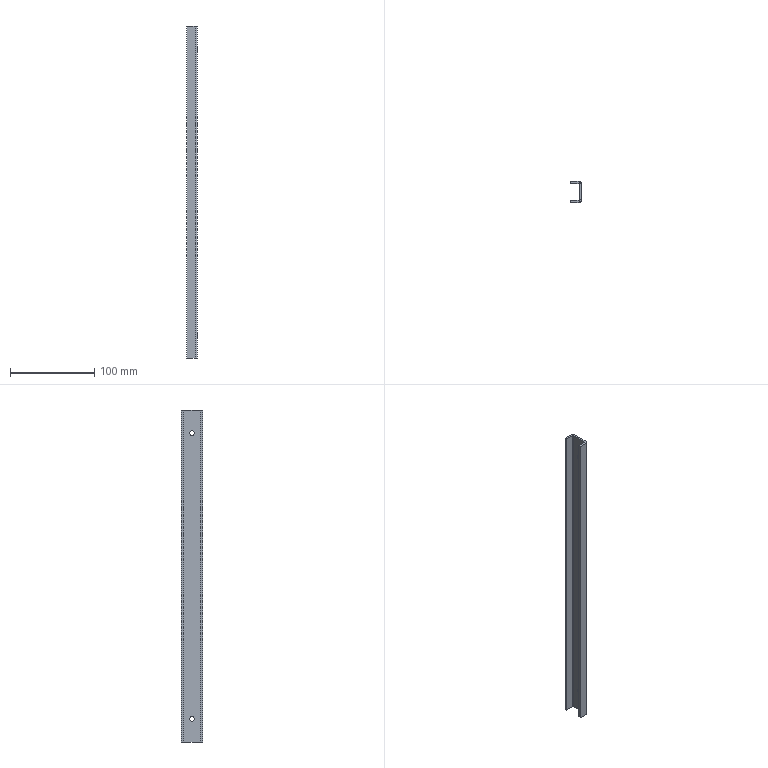Part | SolidWorks | features Cut 1, FlatPattern 1, SMBaseFlange 1, SheetMetal 1 | 1 solid | 26 faces | box 13 x 25 x 395 mm | volume 44005 mm3 | plane 18 | cylinder 8 | commonest cylinder face diameters 5.2 x4 0.6 x2 5.6 x2
STEP:
#1=CARTESIAN_POINT('',(10.5,12.5,30.1));
#2=VERTEX_POINT('',#1);
#3=CARTESIAN_POINT('',(10.5,12.5,24.9));
#4=VERTEX_POINT('',#3);
#5=CARTESIAN_POINT('',(10.5,12.5,27.5));
#6=DIRECTION('',(1.,0.,0.));
#7=DIRECTION('',(0.,0.,-1.));
#8=AXIS2_PLACEMENT_3D('',#5,#6,#7);
#9=CIRCLE('',#8,2.6);
#10=EDGE_CURVE('',#2,#4,#9,.T.);
#11=ORIENTED_EDGE('',*,*,#10,.F.);
#12=CARTESIAN_POINT('',(13.,12.5,30.1));
#13=VERTEX_POINT('',#12);
#14=CARTESIAN_POINT('',(10.5,12.5,30.1));
#15=DIRECTION('',(1.,0.,0.));
#16=VECTOR('',#15,1000.);
#17=LINE('',#14,#16);
#18=EDGE_CURVE('',#2,#13,#17,.T.);
#19=ORIENTED_EDGE('',*,*,#18,.T.);
#20=CARTESIAN_POINT('',(13.,12.5,24.9));
#21=VERTEX_POINT('',#20);
#22=CARTESIAN_POINT('',(13.,12.5,27.5));
#23=DIRECTION('',(1.,0.,0.));
#24=DIRECTION('',(0.,0.,-1.));
#25=AXIS2_PLACEMENT_3D('',#22,#23,#24);
#26=CIRCLE('',#25,2.6);
#27=EDGE_CURVE('',#13,#21,#26,.T.);
#28=ORIENTED_EDGE('',*,*,#27,.T.);
#29=CARTESIAN_POINT('',(10.5,12.5,24.9));
#30=DIRECTION('',(1.,0.,0.));
#31=VECTOR('',#30,1000.);
#32=LINE('',#29,#31);
#33=EDGE_CURVE('',#4,#21,#32,.T.);
#34=ORIENTED_EDGE('',*,*,#33,.F.);
#35=EDGE_LOOP('',(#11,#19,#28,#34));
#36=FACE_OUTER_BOUND('',#35,.T.);
#37=CARTESIAN_POINT('',(10.5,12.5,27.5));
#38=DIRECTION('',(1.,0.,0.));
#39=DIRECTION('',(0.,0.,-1.));
#40=AXIS2_PLACEMENT_3D('',#37,#38,#39);
#41=CYLINDRICAL_SURFACE('',#40,2.6);
#42=ADVANCED_FACE('',(#36),#41,.F.);
#43=CARTESIAN_POINT('',(10.5,12.5,370.1));
#44=VERTEX_POINT('',#43);
#45=CARTESIAN_POINT('',(10.5,12.5,364.9));
#46=VERTEX_POINT('',#45);
#47=CARTESIAN_POINT('',(10.5,12.5,367.5));
#48=DIRECTION('',(1.,0.,0.));
#49=DIRECTION('',(0.,0.,-1.));
#50=AXIS2_PLACEMENT_3D('',#47,#48,#49);
#51=CIRCLE('',#50,2.6);
#52=EDGE_CURVE('',#44,#46,#51,.T.);
#53=ORIENTED_EDGE('',*,*,#52,.F.);
#54=CARTESIAN_POINT('',(13.,12.5,370.1));
#55=VERTEX_POINT('',#54);
#56=CARTESIAN_POINT('',(10.5,12.5,370.1));
#57=DIRECTION('',(1.,0.,0.));
#58=VECTOR('',#57,1000.);
#59=LINE('',#56,#58);
#60=EDGE_CURVE('',#44,#55,#59,.T.);
#61=ORIENTED_EDGE('',*,*,#60,.T.);
#62=CARTESIAN_POINT('',(13.,12.5,364.9));
#63=VERTEX_POINT('',#62);
#64=CARTESIAN_POINT('',(13.,12.5,367.5));
#65=DIRECTION('',(1.,0.,0.));
#66=DIRECTION('',(0.,0.,-1.));
#67=AXIS2_PLACEMENT_3D('',#64,#65,#66);
#68=CIRCLE('',#67,2.6);
#69=EDGE_CURVE('',#55,#63,#68,.T.);
#70=ORIENTED_EDGE('',*,*,#69,.T.);
#71=CARTESIAN_POINT('',(10.5,12.5,364.9));
#72=DIRECTION('',(1.,0.,0.));
#73=VECTOR('',#72,1000.);
#74=LINE('',#71,#73);
#75=EDGE_CURVE('',#46,#63,#74,.T.);
#76=ORIENTED_EDGE('',*,*,#75,.F.);
#77=EDGE_LOOP('',(#53,#61,#70,#76));
#78=FACE_OUTER_BOUND('',#77,.T.);
#79=CARTESIAN_POINT('',(10.5,12.5,367.5));
#80=DIRECTION('',(1.,0.,0.));
#81=DIRECTION('',(0.,0.,-1.));
#82=AXIS2_PLACEMENT_3D('',#79,#80,#81);
#83=CYLINDRICAL_SURFACE('',#82,2.6);
#84=ADVANCED_FACE('',(#78),#83,.F.);
#85=CARTESIAN_POINT('',(10.2,0.,395.));
#86=VERTEX_POINT('',#85);
#87=CARTESIAN_POINT('',(10.2,2.5,395.));
#88=VERTEX_POINT('',#87);
#89=CARTESIAN_POINT('',(10.2,0.,395.));
#90=DIRECTION('',(0.,1.,0.));
#91=VECTOR('',#90,1000.);
#92=LINE('',#89,#91);
#93=EDGE_CURVE('',#86,#88,#92,.T.);
#94=ORIENTED_EDGE('',*,*,#93,.F.);
#95=CARTESIAN_POINT('',(13.,2.8,395.));
#96=VERTEX_POINT('',#95);
#97=CARTESIAN_POINT('',(10.2,2.8,395.));
#98=DIRECTION('',(0.,0.,1.));
#99=DIRECTION('',(-1.,0.,0.));
#100=AXIS2_PLACEMENT_3D('',#97,#98,#99);
#101=CIRCLE('',#100,2.8);
#102=EDGE_CURVE('',#86,#96,#101,.T.);
#103=ORIENTED_EDGE('',*,*,#102,.T.);
#104=CARTESIAN_POINT('',(10.5,2.8,395.));
#105=VERTEX_POINT('',#104);
#106=CARTESIAN_POINT('',(10.5,2.8,395.));
#107=DIRECTION('',(1.,0.,0.));
#108=VECTOR('',#107,1000.);
#109=LINE('',#106,#108);
#110=EDGE_CURVE('',#105,#96,#109,.T.);
#111=ORIENTED_EDGE('',*,*,#110,.F.);
#112=CARTESIAN_POINT('',(10.2,2.8,395.));
#113=DIRECTION('',(0.,0.,1.));
#114=DIRECTION('',(1.,0.,0.));
#115=AXIS2_PLACEMENT_3D('',#112,#113,#114);
#116=CIRCLE('',#115,0.3);
#117=EDGE_CURVE('',#88,#105,#116,.T.);
#118=ORIENTED_EDGE('',*,*,#117,.F.);
#119=EDGE_LOOP('',(#94,#103,#111,#118));
#120=FACE_OUTER_BOUND('',#119,.T.);
#121=CARTESIAN_POINT('',(10.2,0.,395.));
#122=DIRECTION('',(0.,0.,1.));
#123=DIRECTION('',(1.,0.,0.));
#124=AXIS2_PLACEMENT_3D('',#121,#122,#123);
#125=PLANE('',#124);
#126=ADVANCED_FACE('',(#120),#125,.T.);
#127=CARTESIAN_POINT('',(0.,0.,395.));
#128=VERTEX_POINT('',#127);
#129=CARTESIAN_POINT('',(0.,0.,395.));
#130=DIRECTION('',(1.,0.,0.));
#131=VECTOR('',#130,1000.);
#132=LINE('',#129,#131);
#133=EDGE_CURVE('',#128,#86,#132,.T.);
#134=ORIENTED_EDGE('',*,*,#133,.T.);
#135=ORIENTED_EDGE('',*,*,#93,.T.);
#136=CARTESIAN_POINT('',(0.,2.5,395.));
#137=VERTEX_POINT('',#136);
#138=CARTESIAN_POINT('',(0.,2.5,395.));
#139=DIRECTION('',(1.,0.,0.));
#140=VECTOR('',#139,1000.);
#141=LINE('',#138,#140);
#142=EDGE_CURVE('',#137,#88,#141,.T.);
#143=ORIENTED_EDGE('',*,*,#142,.F.);
#144=CARTESIAN_POINT('',(0.,0.,395.));
#145=DIRECTION('',(0.,1.,0.));
#146=VECTOR('',#145,1000.);
#147=LINE('',#144,#146);
#148=EDGE_CURVE('',#128,#137,#147,.T.);
#149=ORIENTED_EDGE('',*,*,#148,.F.);
#150=EDGE_LOOP('',(#134,#135,#143,#149));
#151=FACE_OUTER_BOUND('',#150,.T.);
#152=CARTESIAN_POINT('',(10.5,2.8,395.));
#153=DIRECTION('',(0.,0.,1.));
#154=DIRECTION('',(1.,0.,0.));
#155=AXIS2_PLACEMENT_3D('',#152,#153,#154);
#156=PLANE('',#155);
#157=ADVANCED_FACE('',(#151),#156,.T.);
#158=CARTESIAN_POINT('',(13.,2.8,0.));
#159=VERTEX_POINT('',#158);
#160=CARTESIAN_POINT('',(10.5,2.8,0.));
#161=VERTEX_POINT('',#160);
#162=CARTESIAN_POINT('',(13.,2.8,0.));
#163=DIRECTION('',(-1.,0.,0.));
#164=VECTOR('',#163,1000.);
#165=LINE('',#162,#164);
#166=EDGE_CURVE('',#159,#161,#165,.T.);
#167=ORIENTED_EDGE('',*,*,#166,.F.);
#168=CARTESIAN_POINT('',(10.2,0.,0.));
#169=VERTEX_POINT('',#168);
#170=CARTESIAN_POINT('',(10.2,2.8,0.));
#171=DIRECTION('',(0.,0.,1.));
#172=DIRECTION('',(-1.,0.,0.));
#173=AXIS2_PLACEMENT_3D('',#170,#171,#172);
#174=CIRCLE('',#173,2.8);
#175=EDGE_CURVE('',#169,#159,#174,.T.);
#176=ORIENTED_EDGE('',*,*,#175,.F.);
#177=CARTESIAN_POINT('',(10.2,2.5,0.));
#178=VERTEX_POINT('',#177);
#179=CARTESIAN_POINT('',(10.2,2.5,0.));
#180=DIRECTION('',(0.,-1.,0.));
#181=VECTOR('',#180,1000.);
#182=LINE('',#179,#181);
#183=EDGE_CURVE('',#178,#169,#182,.T.);
#184=ORIENTED_EDGE('',*,*,#183,.F.);
#185=CARTESIAN_POINT('',(10.2,2.8,0.));
#186=DIRECTION('',(0.,0.,1.));
#187=DIRECTION('',(1.,0.,0.));
#188=AXIS2_PLACEMENT_3D('',#185,#186,#187);
#189=CIRCLE('',#188,0.3);
#190=EDGE_CURVE('',#178,#161,#189,.T.);
#191=ORIENTED_EDGE('',*,*,#190,.T.);
#192=EDGE_LOOP('',(#167,#176,#184,#191));
#193=FACE_OUTER_BOUND('',#192,.T.);
#194=CARTESIAN_POINT('',(13.,2.8,0.));
#195=DIRECTION('',(0.,0.,-1.));
#196=DIRECTION('',(-1.,0.,0.));
#197=AXIS2_PLACEMENT_3D('',#194,#195,#196);
#198=PLANE('',#197);
#199=ADVANCED_FACE('',(#193),#198,.T.);
#200=CARTESIAN_POINT('',(13.,22.2,0.));
#201=VERTEX_POINT('',#200);
#202=CARTESIAN_POINT('',(13.,0.,0.));
#203=DIRECTION('',(0.,1.,0.));
#204=VECTOR('',#203,1000.);
#205=LINE('',#202,#204);
#206=EDGE_CURVE('',#159,#201,#205,.T.);
#207=ORIENTED_EDGE('',*,*,#206,.F.);
#208=ORIENTED_EDGE('',*,*,#166,.T.);
#209=CARTESIAN_POINT('',(10.5,22.2,0.));
#210=VERTEX_POINT('',#209);
#211=CARTESIAN_POINT('',(10.5,0.,0.));
#212=DIRECTION('',(0.,1.,0.));
#213=VECTOR('',#212,1000.);
#214=LINE('',#211,#213);
#215=EDGE_CURVE('',#161,#210,#214,.T.);
#216=ORIENTED_EDGE('',*,*,#215,.T.);
#217=CARTESIAN_POINT('',(10.5,22.2,0.));
#218=DIRECTION('',(1.,0.,0.));
#219=VECTOR('',#218,1000.);
#220=LINE('',#217,#219);
#221=EDGE_CURVE('',#210,#201,#220,.T.);
#222=ORIENTED_EDGE('',*,*,#221,.T.);
#223=EDGE_LOOP('',(#207,#208,#216,#222));
#224=FACE_OUTER_BOUND('',#223,.T.);
#225=CARTESIAN_POINT('',(10.2,2.5,0.));
#226=DIRECTION('',(0.,0.,-1.));
#227=DIRECTION('',(-1.,0.,0.));
#228=AXIS2_PLACEMENT_3D('',#225,#226,#227);
#229=PLANE('',#228);
#230=ADVANCED_FACE('',(#224),#229,.T.);
#231=CARTESIAN_POINT('',(13.,22.2,395.));
#232=VERTEX_POINT('',#231);
#233=CARTESIAN_POINT('',(10.5,22.2,395.));
#234=VERTEX_POINT('',#233);
#235=CARTESIAN_POINT('',(13.,22.2,395.));
#236=DIRECTION('',(-1.,0.,0.));
#237=VECTOR('',#236,1000.);
#238=LINE('',#235,#237);
#239=EDGE_CURVE('',#232,#234,#238,.T.);
#240=ORIENTED_EDGE('',*,*,#239,.F.);
#241=CARTESIAN_POINT('',(10.2,25.,395.));
#242=VERTEX_POINT('',#241);
#243=CARTESIAN_POINT('',(10.2,22.2,395.));
#244=DIRECTION('',(0.,0.,1.));
#245=DIRECTION('',(-1.,0.,0.));
#246=AXIS2_PLACEMENT_3D('',#243,#244,#245);
#247=CIRCLE('',#246,2.8);
#248=EDGE_CURVE('',#232,#242,#247,.T.);
#249=ORIENTED_EDGE('',*,*,#248,.T.);
#250=CARTESIAN_POINT('',(10.2,22.5,395.));
#251=VERTEX_POINT('',#250);
#252=CARTESIAN_POINT('',(10.2,22.5,395.));
#253=DIRECTION('',(0.,1.,0.));
#254=VECTOR('',#253,1000.);
#255=LINE('',#252,#254);
#256=EDGE_CURVE('',#251,#242,#255,.T.);
#257=ORIENTED_EDGE('',*,*,#256,.F.);
#258=CARTESIAN_POINT('',(10.2,22.2,395.));
#259=DIRECTION('',(0.,0.,1.));
#260=DIRECTION('',(1.,0.,0.));
#261=AXIS2_PLACEMENT_3D('',#258,#259,#260);
#262=CIRCLE('',#261,0.3);
#263=EDGE_CURVE('',#234,#251,#262,.T.);
#264=ORIENTED_EDGE('',*,*,#263,.F.);
#265=EDGE_LOOP('',(#240,#249,#257,#264));
#266=FACE_OUTER_BOUND('',#265,.T.);
#267=CARTESIAN_POINT('',(13.,22.2,395.));
#268=DIRECTION('',(0.,0.,1.));
#269=DIRECTION('',(1.,0.,0.));
#270=AXIS2_PLACEMENT_3D('',#267,#268,#269);
#271=PLANE('',#270);
#272=ADVANCED_FACE('',(#266),#271,.T.);
#273=CARTESIAN_POINT('',(13.,0.,395.));
#274=DIRECTION('',(0.,1.,0.));
#275=VECTOR('',#274,1000.);
#276=LINE('',#273,#275);
#277=EDGE_CURVE('',#96,#232,#276,.T.);
#278=ORIENTED_EDGE('',*,*,#277,.T.);
#279=ORIENTED_EDGE('',*,*,#239,.T.);
#280=CARTESIAN_POINT('',(10.5,0.,395.));
#281=DIRECTION('',(0.,1.,0.));
#282=VECTOR('',#281,1000.);
#283=LINE('',#280,#282);
#284=EDGE_CURVE('',#105,#234,#283,.T.);
#285=ORIENTED_EDGE('',*,*,#284,.F.);
#286=ORIENTED_EDGE('',*,*,#110,.T.);
#287=EDGE_LOOP('',(#278,#279,#285,#286));
#288=FACE_OUTER_BOUND('',#287,.T.);
#289=CARTESIAN_POINT('',(10.2,22.5,395.));
#290=DIRECTION('',(0.,0.,1.));
#291=DIRECTION('',(1.,0.,0.));
#292=AXIS2_PLACEMENT_3D('',#289,#290,#291);
#293=PLANE('',#292);
#294=ADVANCED_FACE('',(#288),#293,.T.);
#295=CARTESIAN_POINT('',(10.2,25.,0.));
#296=VERTEX_POINT('',#295);
#297=CARTESIAN_POINT('',(10.2,22.5,0.));
#298=VERTEX_POINT('',#297);
#299=CARTESIAN_POINT('',(10.2,25.,0.));
#300=DIRECTION('',(0.,-1.,0.));
#301=VECTOR('',#300,1000.);
#302=LINE('',#299,#301);
#303=EDGE_CURVE('',#296,#298,#302,.T.);
#304=ORIENTED_EDGE('',*,*,#303,.F.);
#305=CARTESIAN_POINT('',(10.2,22.2,0.));
#306=DIRECTION('',(0.,0.,1.));
#307=DIRECTION('',(-1.,0.,0.));
#308=AXIS2_PLACEMENT_3D('',#305,#306,#307);
#309=CIRCLE('',#308,2.8);
#310=EDGE_CURVE('',#201,#296,#309,.T.);
#311=ORIENTED_EDGE('',*,*,#310,.F.);
#312=ORIENTED_EDGE('',*,*,#221,.F.);
#313=CARTESIAN_POINT('',(10.2,22.2,0.));
#314=DIRECTION('',(0.,0.,1.));
#315=DIRECTION('',(1.,0.,0.));
#316=AXIS2_PLACEMENT_3D('',#313,#314,#315);
#317=CIRCLE('',#316,0.3);
#318=EDGE_CURVE('',#210,#298,#317,.T.);
#319=ORIENTED_EDGE('',*,*,#318,.T.);
#320=EDGE_LOOP('',(#304,#311,#312,#319));
#321=FACE_OUTER_BOUND('',#320,.T.);
#322=CARTESIAN_POINT('',(10.2,25.,0.));
#323=DIRECTION('',(0.,0.,-1.));
#324=DIRECTION('',(-1.,0.,0.));
#325=AXIS2_PLACEMENT_3D('',#322,#323,#324);
#326=PLANE('',#325);
#327=ADVANCED_FACE('',(#321),#326,.T.);
#328=CARTESIAN_POINT('',(0.,25.,0.));
#329=VERTEX_POINT('',#328);
#330=CARTESIAN_POINT('',(13.,25.,0.));
#331=DIRECTION('',(-1.,0.,0.));
#332=VECTOR('',#331,1000.);
#333=LINE('',#330,#332);
#334=EDGE_CURVE('',#296,#329,#333,.T.);
#335=ORIENTED_EDGE('',*,*,#334,.F.);
#336=ORIENTED_EDGE('',*,*,#303,.T.);
#337=CARTESIAN_POINT('',(0.,22.5,0.));
#338=VERTEX_POINT('',#337);
#339=CARTESIAN_POINT('',(13.,22.5,0.));
#340=DIRECTION('',(-1.,0.,0.));
#341=VECTOR('',#340,1000.);
#342=LINE('',#339,#341);
#343=EDGE_CURVE('',#298,#338,#342,.T.);
#344=ORIENTED_EDGE('',*,*,#343,.T.);
#345=CARTESIAN_POINT('',(0.,22.5,0.));
#346=DIRECTION('',(0.,1.,0.));
#347=VECTOR('',#346,1000.);
#348=LINE('',#345,#347);
#349=EDGE_CURVE('',#338,#329,#348,.T.);
#350=ORIENTED_EDGE('',*,*,#349,.T.);
#351=EDGE_LOOP('',(#335,#336,#344,#350));
#352=FACE_OUTER_BOUND('',#351,.T.);
#353=CARTESIAN_POINT('',(10.5,22.2,0.));
#354=DIRECTION('',(0.,0.,-1.));
#355=DIRECTION('',(-1.,0.,0.));
#356=AXIS2_PLACEMENT_3D('',#353,#354,#355);
#357=PLANE('',#356);
#358=ADVANCED_FACE('',(#352),#357,.T.);
#359=ORIENTED_EDGE('',*,*,#334,.T.);
#360=CARTESIAN_POINT('',(0.,25.,395.));
#361=VERTEX_POINT('',#360);
#362=CARTESIAN_POINT('',(0.,25.,395.));
#363=DIRECTION('',(0.,0.,-1.));
#364=VECTOR('',#363,1000.);
#365=LINE('',#362,#364);
#366=EDGE_CURVE('',#361,#329,#365,.T.);
#367=ORIENTED_EDGE('',*,*,#366,.F.);
#368=CARTESIAN_POINT('',(13.,25.,395.));
#369=DIRECTION('',(-1.,0.,0.));
#370=VECTOR('',#369,1000.);
#371=LINE('',#368,#370);
#372=EDGE_CURVE('',#242,#361,#371,.T.);
#373=ORIENTED_EDGE('',*,*,#372,.F.);
#374=CARTESIAN_POINT('',(10.2,25.,395.));
#375=DIRECTION('',(0.,0.,-1.));
#376=VECTOR('',#375,1000.);
#377=LINE('',#374,#376);
#378=EDGE_CURVE('',#242,#296,#377,.T.);
#379=ORIENTED_EDGE('',*,*,#378,.T.);
#380=EDGE_LOOP('',(#359,#367,#373,#379));
#381=FACE_OUTER_BOUND('',#380,.T.);
#382=CARTESIAN_POINT('',(13.,25.,395.));
#383=DIRECTION('',(0.,-1.,0.));
#384=DIRECTION('',(0.,0.,-1.));
#385=AXIS2_PLACEMENT_3D('',#382,#383,#384);
#386=PLANE('',#385);
#387=ADVANCED_FACE('',(#381),#386,.F.);
#388=ORIENTED_EDGE('',*,*,#349,.F.);
#389=CARTESIAN_POINT('',(0.,22.5,395.));
#390=VERTEX_POINT('',#389);
#391=CARTESIAN_POINT('',(0.,22.5,395.));
#392=DIRECTION('',(0.,0.,-1.));
#393=VECTOR('',#392,1000.);
#394=LINE('',#391,#393);
#395=EDGE_CURVE('',#390,#338,#394,.T.);
#396=ORIENTED_EDGE('',*,*,#395,.F.);
#397=CARTESIAN_POINT('',(0.,22.5,395.));
#398=DIRECTION('',(0.,1.,0.));
#399=VECTOR('',#398,1000.);
#400=LINE('',#397,#399);
#401=EDGE_CURVE('',#390,#361,#400,.T.);
#402=ORIENTED_EDGE('',*,*,#401,.T.);
#403=ORIENTED_EDGE('',*,*,#366,.T.);
#404=EDGE_LOOP('',(#388,#396,#402,#403));
#405=FACE_OUTER_BOUND('',#404,.T.);
#406=CARTESIAN_POINT('',(0.,22.5,395.));
#407=DIRECTION('',(-1.,0.,0.));
#408=DIRECTION('',(0.,0.,1.));
#409=AXIS2_PLACEMENT_3D('',#406,#407,#408);
#410=PLANE('',#409);
#411=ADVANCED_FACE('',(#405),#410,.T.);
#412=ORIENTED_EDGE('',*,*,#343,.F.);
#413=CARTESIAN_POINT('',(10.2,22.5,395.));
#414=DIRECTION('',(0.,0.,-1.));
#415=VECTOR('',#414,1000.);
#416=LINE('',#413,#415);
#417=EDGE_CURVE('',#251,#298,#416,.T.);
#418=ORIENTED_EDGE('',*,*,#417,.F.);
#419=CARTESIAN_POINT('',(13.,22.5,395.));
#420=DIRECTION('',(-1.,0.,0.));
#421=VECTOR('',#420,1000.);
#422=LINE('',#419,#421);
#423=EDGE_CURVE('',#251,#390,#422,.T.);
#424=ORIENTED_EDGE('',*,*,#423,.T.);
#425=ORIENTED_EDGE('',*,*,#395,.T.);
#426=EDGE_LOOP('',(#412,#418,#424,#425));
#427=FACE_OUTER_BOUND('',#426,.T.);
#428=CARTESIAN_POINT('',(13.,22.5,395.));
#429=DIRECTION('',(0.,-1.,0.));
#430=DIRECTION('',(0.,0.,-1.));
#431=AXIS2_PLACEMENT_3D('',#428,#429,#430);
#432=PLANE('',#431);
#433=ADVANCED_FACE('',(#427),#432,.T.);
#434=ORIENTED_EDGE('',*,*,#318,.F.);
#435=CARTESIAN_POINT('',(10.5,22.2,395.));
#436=DIRECTION('',(0.,0.,-1.));
#437=VECTOR('',#436,1000.);
#438=LINE('',#435,#437);
#439=EDGE_CURVE('',#234,#210,#438,.T.);
#440=ORIENTED_EDGE('',*,*,#439,.F.);
#441=ORIENTED_EDGE('',*,*,#263,.T.);
#442=ORIENTED_EDGE('',*,*,#417,.T.);
#443=EDGE_LOOP('',(#434,#440,#441,#442));
#444=FACE_OUTER_BOUND('',#443,.T.);
#445=CARTESIAN_POINT('',(10.2,22.2,395.));
#446=DIRECTION('',(0.,0.,-1.));
#447=DIRECTION('',(-1.,0.,0.));
#448=AXIS2_PLACEMENT_3D('',#445,#446,#447);
#449=CYLINDRICAL_SURFACE('',#448,0.3);
#450=ADVANCED_FACE('',(#444),#449,.F.);
#451=CARTESIAN_POINT('',(10.5,12.5,27.5));
#452=DIRECTION('',(1.,0.,0.));
#453=DIRECTION('',(0.,0.,-1.));
#454=AXIS2_PLACEMENT_3D('',#451,#452,#453);
#455=CIRCLE('',#454,2.6);
#456=EDGE_CURVE('',#4,#2,#455,.T.);
#457=ORIENTED_EDGE('',*,*,#456,.T.);
#458=ORIENTED_EDGE('',*,*,#10,.T.);
#459=EDGE_LOOP('',(#457,#458));
#460=FACE_BOUND('',#459,.T.);
#461=CARTESIAN_POINT('',(10.5,12.5,367.5));
#462=DIRECTION('',(1.,0.,0.));
#463=DIRECTION('',(0.,0.,-1.));
#464=AXIS2_PLACEMENT_3D('',#461,#462,#463);
#465=CIRCLE('',#464,2.6);
#466=EDGE_CURVE('',#46,#44,#465,.T.);
#467=ORIENTED_EDGE('',*,*,#466,.T.);
#468=ORIENTED_EDGE('',*,*,#52,.T.);
#469=EDGE_LOOP('',(#467,#468));
#470=FACE_BOUND('',#469,.T.);
#471=ORIENTED_EDGE('',*,*,#215,.F.);
#472=CARTESIAN_POINT('',(10.5,2.8,395.));
#473=DIRECTION('',(0.,0.,-1.));
#474=VECTOR('',#473,1000.);
#475=LINE('',#472,#474);
#476=EDGE_CURVE('',#105,#161,#475,.T.);
#477=ORIENTED_EDGE('',*,*,#476,.F.);
#478=ORIENTED_EDGE('',*,*,#284,.T.);
#479=ORIENTED_EDGE('',*,*,#439,.T.);
#480=EDGE_LOOP('',(#471,#477,#478,#479));
#481=FACE_OUTER_BOUND('',#480,.T.);
#482=CARTESIAN_POINT('',(10.5,0.,395.));
#483=DIRECTION('',(-1.,0.,0.));
#484=DIRECTION('',(0.,0.,1.));
#485=AXIS2_PLACEMENT_3D('',#482,#483,#484);
#486=PLANE('',#485);
#487=ADVANCED_FACE('',(#460,#470,#481),#486,.T.);
#488=ORIENTED_EDGE('',*,*,#190,.F.);
#489=CARTESIAN_POINT('',(10.2,2.5,395.));
#490=DIRECTION('',(0.,0.,-1.));
#491=VECTOR('',#490,1000.);
#492=LINE('',#489,#491);
#493=EDGE_CURVE('',#88,#178,#492,.T.);
#494=ORIENTED_EDGE('',*,*,#493,.F.);
#495=ORIENTED_EDGE('',*,*,#117,.T.);
#496=ORIENTED_EDGE('',*,*,#476,.T.);
#497=EDGE_LOOP('',(#488,#494,#495,#496));
#498=FACE_OUTER_BOUND('',#497,.T.);
#499=CARTESIAN_POINT('',(10.2,2.8,395.));
#500=DIRECTION('',(0.,0.,-1.));
#501=DIRECTION('',(-1.,0.,0.));
#502=AXIS2_PLACEMENT_3D('',#499,#500,#501);
#503=CYLINDRICAL_SURFACE('',#502,0.3);
#504=ADVANCED_FACE('',(#498),#503,.F.);
#505=CARTESIAN_POINT('',(0.,2.5,0.));
#506=VERTEX_POINT('',#505);
#507=CARTESIAN_POINT('',(0.,2.5,0.));
#508=DIRECTION('',(1.,0.,0.));
#509=VECTOR('',#508,1000.);
#510=LINE('',#507,#509);
#511=EDGE_CURVE('',#506,#178,#510,.T.);
#512=ORIENTED_EDGE('',*,*,#511,.F.);
#513=CARTESIAN_POINT('',(0.,2.5,395.));
#514=DIRECTION('',(0.,0.,-1.));
#515=VECTOR('',#514,1000.);
#516=LINE('',#513,#515);
#517=EDGE_CURVE('',#137,#506,#516,.T.);
#518=ORIENTED_EDGE('',*,*,#517,.F.);
#519=ORIENTED_EDGE('',*,*,#142,.T.);
#520=ORIENTED_EDGE('',*,*,#493,.T.);
#521=EDGE_LOOP('',(#512,#518,#519,#520));
#522=FACE_OUTER_BOUND('',#521,.T.);
#523=CARTESIAN_POINT('',(0.,2.5,395.));
#524=DIRECTION('',(0.,1.,0.));
#525=DIRECTION('',(0.,0.,1.));
#526=AXIS2_PLACEMENT_3D('',#523,#524,#525);
#527=PLANE('',#526);
#528=ADVANCED_FACE('',(#522),#527,.T.);
#529=CARTESIAN_POINT('',(0.,0.,0.));
#530=VERTEX_POINT('',#529);
#531=CARTESIAN_POINT('',(0.,0.,0.));
#532=DIRECTION('',(0.,1.,0.));
#533=VECTOR('',#532,1000.);
#534=LINE('',#531,#533);
#535=EDGE_CURVE('',#530,#506,#534,.T.);
#536=ORIENTED_EDGE('',*,*,#535,.F.);
#537=CARTESIAN_POINT('',(0.,0.,395.));
#538=DIRECTION('',(0.,0.,-1.));
#539=VECTOR('',#538,1000.);
#540=LINE('',#537,#539);
#541=EDGE_CURVE('',#128,#530,#540,.T.);
#542=ORIENTED_EDGE('',*,*,#541,.F.);
#543=ORIENTED_EDGE('',*,*,#148,.T.);
#544=ORIENTED_EDGE('',*,*,#517,.T.);
#545=EDGE_LOOP('',(#536,#542,#543,#544));
#546=FACE_OUTER_BOUND('',#545,.T.);
#547=CARTESIAN_POINT('',(0.,0.,395.));
#548=DIRECTION('',(-1.,0.,0.));
#549=DIRECTION('',(0.,0.,1.));
#550=AXIS2_PLACEMENT_3D('',#547,#548,#549);
#551=PLANE('',#550);
#552=ADVANCED_FACE('',(#546),#551,.T.);
#553=CARTESIAN_POINT('',(0.,0.,0.));
#554=DIRECTION('',(1.,0.,0.));
#555=VECTOR('',#554,1000.);
#556=LINE('',#553,#555);
#557=EDGE_CURVE('',#530,#169,#556,.T.);
#558=ORIENTED_EDGE('',*,*,#557,.T.);
#559=CARTESIAN_POINT('',(10.2,0.,395.));
#560=DIRECTION('',(0.,0.,-1.));
#561=VECTOR('',#560,1000.);
#562=LINE('',#559,#561);
#563=EDGE_CURVE('',#86,#169,#562,.T.);
#564=ORIENTED_EDGE('',*,*,#563,.F.);
#565=ORIENTED_EDGE('',*,*,#133,.F.);
#566=ORIENTED_EDGE('',*,*,#541,.T.);
#567=EDGE_LOOP('',(#558,#564,#565,#566));
#568=FACE_OUTER_BOUND('',#567,.T.);
#569=CARTESIAN_POINT('',(0.,0.,395.));
#570=DIRECTION('',(0.,1.,0.));
#571=DIRECTION('',(0.,0.,1.));
#572=AXIS2_PLACEMENT_3D('',#569,#570,#571);
#573=PLANE('',#572);
#574=ADVANCED_FACE('',(#568),#573,.F.);
#575=ORIENTED_EDGE('',*,*,#175,.T.);
#576=CARTESIAN_POINT('',(13.,2.8,395.));
#577=DIRECTION('',(0.,0.,-1.));
#578=VECTOR('',#577,1000.);
#579=LINE('',#576,#578);
#580=EDGE_CURVE('',#96,#159,#579,.T.);
#581=ORIENTED_EDGE('',*,*,#580,.F.);
#582=ORIENTED_EDGE('',*,*,#102,.F.);
#583=ORIENTED_EDGE('',*,*,#563,.T.);
#584=EDGE_LOOP('',(#575,#581,#582,#583));
#585=FACE_OUTER_BOUND('',#584,.T.);
#586=CARTESIAN_POINT('',(10.2,2.8,395.));
#587=DIRECTION('',(0.,0.,-1.));
#588=DIRECTION('',(-1.,0.,0.));
#589=AXIS2_PLACEMENT_3D('',#586,#587,#588);
#590=CYLINDRICAL_SURFACE('',#589,2.8);
#591=ADVANCED_FACE('',(#585),#590,.T.);
#592=CARTESIAN_POINT('',(13.,12.5,27.5));
#593=DIRECTION('',(1.,0.,0.));
#594=DIRECTION('',(0.,0.,-1.));
#595=AXIS2_PLACEMENT_3D('',#592,#593,#594);
#596=CIRCLE('',#595,2.6);
#597=EDGE_CURVE('',#21,#13,#596,.T.);
#598=ORIENTED_EDGE('',*,*,#597,.F.);
#599=ORIENTED_EDGE('',*,*,#27,.F.);
#600=EDGE_LOOP('',(#598,#599));
#601=FACE_BOUND('',#600,.T.);
#602=CARTESIAN_POINT('',(13.,12.5,367.5));
#603=DIRECTION('',(1.,0.,0.));
#604=DIRECTION('',(0.,0.,-1.));
#605=AXIS2_PLACEMENT_3D('',#602,#603,#604);
#606=CIRCLE('',#605,2.6);
#607=EDGE_CURVE('',#63,#55,#606,.T.);
#608=ORIENTED_EDGE('',*,*,#607,.F.);
#609=ORIENTED_EDGE('',*,*,#69,.F.);
#610=EDGE_LOOP('',(#608,#609));
#611=FACE_BOUND('',#610,.T.);
#612=ORIENTED_EDGE('',*,*,#206,.T.);
#613=CARTESIAN_POINT('',(13.,22.2,395.));
#614=DIRECTION('',(0.,0.,-1.));
#615=VECTOR('',#614,1000.);
#616=LINE('',#613,#615);
#617=EDGE_CURVE('',#232,#201,#616,.T.);
#618=ORIENTED_EDGE('',*,*,#617,.F.);
#619=ORIENTED_EDGE('',*,*,#277,.F.);
#620=ORIENTED_EDGE('',*,*,#580,.T.);
#621=EDGE_LOOP('',(#612,#618,#619,#620));
#622=FACE_OUTER_BOUND('',#621,.T.);
#623=CARTESIAN_POINT('',(13.,0.,395.));
#624=DIRECTION('',(-1.,0.,0.));
#625=DIRECTION('',(0.,0.,1.));
#626=AXIS2_PLACEMENT_3D('',#623,#624,#625);
#627=PLANE('',#626);
#628=ADVANCED_FACE('',(#601,#611,#622),#627,.F.);
#629=ORIENTED_EDGE('',*,*,#310,.T.);
#630=ORIENTED_EDGE('',*,*,#378,.F.);
#631=ORIENTED_EDGE('',*,*,#248,.F.);
#632=ORIENTED_EDGE('',*,*,#617,.T.);
#633=EDGE_LOOP('',(#629,#630,#631,#632));
#634=FACE_OUTER_BOUND('',#633,.T.);
#635=CARTESIAN_POINT('',(10.2,22.2,395.));
#636=DIRECTION('',(0.,0.,-1.));
#637=DIRECTION('',(-1.,0.,0.));
#638=AXIS2_PLACEMENT_3D('',#635,#636,#637);
#639=CYLINDRICAL_SURFACE('',#638,2.8);
#640=ADVANCED_FACE('',(#634),#639,.T.);
#641=ORIENTED_EDGE('',*,*,#372,.T.);
#642=ORIENTED_EDGE('',*,*,#401,.F.);
#643=ORIENTED_EDGE('',*,*,#423,.F.);
#644=ORIENTED_EDGE('',*,*,#256,.T.);
#645=EDGE_LOOP('',(#641,#642,#643,#644));
#646=FACE_OUTER_BOUND('',#645,.T.);
#647=CARTESIAN_POINT('',(10.2,22.2,395.));
#648=DIRECTION('',(0.,0.,1.));
#649=DIRECTION('',(1.,0.,0.));
#650=AXIS2_PLACEMENT_3D('',#647,#648,#649);
#651=PLANE('',#650);
#652=ADVANCED_FACE('',(#646),#651,.T.);
#653=ORIENTED_EDGE('',*,*,#511,.T.);
#654=ORIENTED_EDGE('',*,*,#183,.T.);
#655=ORIENTED_EDGE('',*,*,#557,.F.);
#656=ORIENTED_EDGE('',*,*,#535,.T.);
#657=EDGE_LOOP('',(#653,#654,#655,#656));
#658=FACE_OUTER_BOUND('',#657,.T.);
#659=CARTESIAN_POINT('',(10.2,22.2,0.));
#660=DIRECTION('',(0.,0.,1.));
#661=DIRECTION('',(1.,0.,0.));
#662=AXIS2_PLACEMENT_3D('',#659,#660,#661);
#663=PLANE('',#662);
#664=ADVANCED_FACE('',(#658),#663,.F.);
#665=ORIENTED_EDGE('',*,*,#60,.F.);
#666=ORIENTED_EDGE('',*,*,#466,.F.);
#667=ORIENTED_EDGE('',*,*,#75,.T.);
#668=ORIENTED_EDGE('',*,*,#607,.T.);
#669=EDGE_LOOP('',(#665,#666,#667,#668));
#670=FACE_OUTER_BOUND('',#669,.T.);
#671=CARTESIAN_POINT('',(10.5,12.5,367.5));
#672=DIRECTION('',(1.,0.,0.));
#673=DIRECTION('',(0.,0.,-1.));
#674=AXIS2_PLACEMENT_3D('',#671,#672,#673);
#675=CYLINDRICAL_SURFACE('',#674,2.6);
#676=ADVANCED_FACE('',(#670),#675,.F.);
#677=ORIENTED_EDGE('',*,*,#18,.F.);
#678=ORIENTED_EDGE('',*,*,#456,.F.);
#679=ORIENTED_EDGE('',*,*,#33,.T.);
#680=ORIENTED_EDGE('',*,*,#597,.T.);
#681=EDGE_LOOP('',(#677,#678,#679,#680));
#682=FACE_OUTER_BOUND('',#681,.T.);
#683=CARTESIAN_POINT('',(10.5,12.5,27.5));
#684=DIRECTION('',(1.,0.,0.));
#685=DIRECTION('',(0.,0.,-1.));
#686=AXIS2_PLACEMENT_3D('',#683,#684,#685);
#687=CYLINDRICAL_SURFACE('',#686,2.6);
#688=ADVANCED_FACE('',(#682),#687,.F.);
#689=CLOSED_SHELL('',(#42,#84,#126,#157,#199,#230,#272,#294,#327,#358,#387,#411,#433,#450,#487,#504,#528,#552,#574,#591,#628,#640,#652,#664,#676,#688));
#690=MANIFOLD_SOLID_BREP('',#689);
#691=CARTESIAN_POINT('',(0.,0.,0.));
#692=DIRECTION('',(0.,0.,1.));
#693=DIRECTION('',(1.,0.,0.));
#694=AXIS2_PLACEMENT_3D('',#691,#692,#693);
#695=(LENGTH_UNIT()NAMED_UNIT(*)SI_UNIT(.MILLI.,.METRE.));
#696=UNCERTAINTY_MEASURE_WITH_UNIT(LENGTH_MEASURE(0.00001),#695,'','');
#697=(NAMED_UNIT(*)PLANE_ANGLE_UNIT()SI_UNIT($,.RADIAN.));
#698=(NAMED_UNIT(*)SI_UNIT($,.STERADIAN.)SOLID_ANGLE_UNIT());
#699=(GEOMETRIC_REPRESENTATION_CONTEXT(3)GLOBAL_UNCERTAINTY_ASSIGNED_CONTEXT((#696))GLOBAL_UNIT_ASSIGNED_CONTEXT((#695,#697,#698))REPRESENTATION_CONTEXT('',''));
#700=ADVANCED_BREP_SHAPE_REPRESENTATION('',(#690,#694),#699);